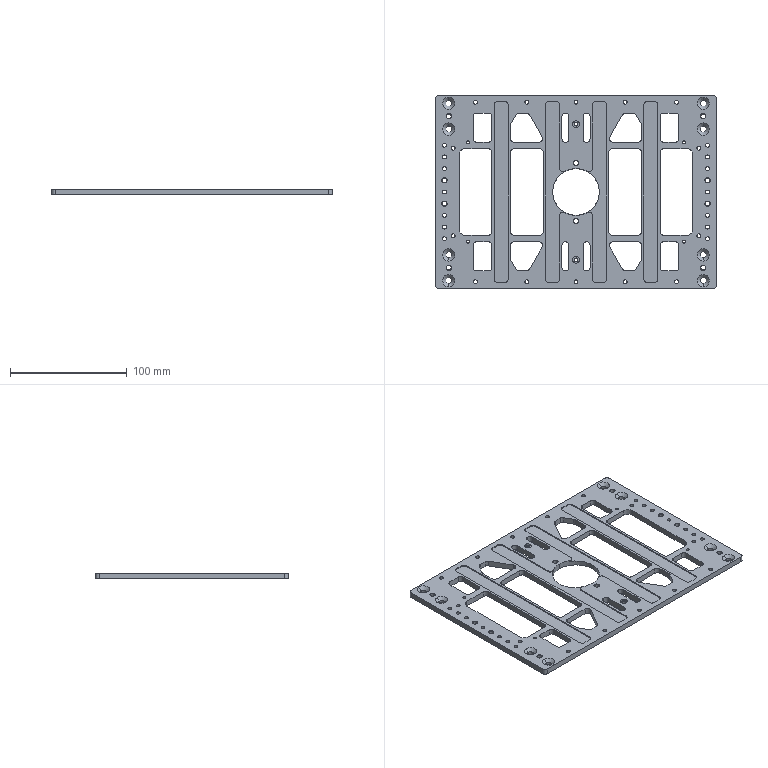NC program | NX | posted with a generic post | part box 240 x 165 x 5 mm
Lines 1759 to 2596 of 12487:
(ZLEVEL_PROFILE_COPY_COPY_1 , TOOL : D4)
N3450 T11 M6
N3452 G54
N3454 G17 G0 G90 X-10. Y-63.427 S9500 M3
N3456 G43 Z30. H11
N3458 Z1.5
N3460 G94 G1 Y-64.672 Z1.435 F1000.
N3462 X-9.86 Y-65.067 Z1.413
N3464 X-9.333 Y-65.475 Z1.378
N3466 X-8.666 Y-65.474 Z1.343
N3468 X-8.251 Y-65.207 Z1.317
N3470 X-8. Y-64.747 Z1.29
N3472 Y-45.253 Z0.268
N3474 X-8.267 Y-44.776 Z0.239
N3476 X-8.741 Y-44.503 Z0.211
N3478 X-9.235 Y-44.497 Z0.185
N3480 X-9.724 Y-44.767 Z0.155
N3482 X-10. Y-45.253 Z0.126
N3484 Y-55. Z-0.385
N3486 Y-64.5 F1800.
N3488 G3 X-9. Y-65.5 R1.
N3490 X-8. Y-64.5 R1.
N3492 G1 Y-45.5
N3494 G3 X-9. Y-44.5 R1.
N3496 X-10. Y-45.5 R1.
N3498 G1 Y-55.
N3500 Y-62.917 Z-0.453
N3502 X-9.983 Y-64.5 Z-0.467
N3504 X-9.955 Y-64.723 Z-0.469
N3506 X-9.921 Y-64.827 Z-0.47
N3508 X-9.782 Y-65.083 Z-0.473
N3510 X-9.691 Y-65.2 Z-0.474
N3512 X-9.501 Y-65.346 Z-0.476
N3514 X-9.316 Y-65.425 Z-0.478
N3516 X-9.063 Y-65.476 Z-0.48
N3518 X-8.881 Y-65.468 Z-0.482
N3520 X-8.635 Y-65.405 Z-0.484
N3522 X-8.47 Y-65.323 Z-0.486
N3524 X-8.336 Y-65.221 Z-0.487
N3526 X-8.233 Y-65.103 Z-0.489
N3528 X-8.127 Y-64.94 Z-0.49
N3530 X-8.076 Y-64.819 Z-0.491
N3532 X-8.039 Y-64.676 Z-0.493
N3534 X-8.017 Y-64.5 Z-0.494
N3536 X-8. Y-62.6 Z-0.511
N3538 Y-47.4 Z-0.643
N3540 X-8.017 Y-45.5 Z-0.66
N3542 X-8.047 Y-45.262 Z-0.662
N3544 X-8.097 Y-45.129 Z-0.663
N3546 X-8.219 Y-44.915 Z-0.665
N3548 X-8.301 Y-44.809 Z-0.666
N3550 X-8.474 Y-44.649 Z-0.668
N3552 X-8.609 Y-44.58 Z-0.67
N3554 X-8.988 Y-44.5 Z-0.673
N3556 X-9.145 Y-44.535 Z-0.674
N3558 X-9.365 Y-44.595 Z-0.676
N3560 X-9.566 Y-44.705 Z-0.678
N3562 X-9.691 Y-44.801 Z-0.68
N3564 X-9.812 Y-44.955 Z-0.682
N3566 X-9.9 Y-45.124 Z-0.683
N3568 X-9.956 Y-45.287 Z-0.685
N3570 X-9.983 Y-45.5 Z-0.687
N3572 X-10. Y-47.083 Z-0.7
N3574 Y-55. Z-0.769
N3576 Y-62.917 Z-0.838
N3578 X-9.983 Y-64.5 Z-0.852
N3580 X-9.955 Y-64.723 Z-0.854
N3582 X-9.921 Y-64.827 Z-0.855
N3584 X-9.782 Y-65.083 Z-0.857
N3586 X-9.691 Y-65.2 Z-0.859
N3588 X-9.501 Y-65.346 Z-0.861
N3590 X-9.316 Y-65.425 Z-0.863
N3592 X-9.063 Y-65.476 Z-0.865
N3594 X-8.881 Y-65.468 Z-0.866
N3596 X-8.635 Y-65.405 Z-0.869
N3598 X-8.47 Y-65.323 Z-0.87
N3600 X-8.336 Y-65.221 Z-0.872
N3602 X-8.233 Y-65.103 Z-0.873
N3604 X-8.127 Y-64.94 Z-0.875
N3606 X-8.076 Y-64.819 Z-0.876
N3608 X-8.039 Y-64.676 Z-0.877
N3610 X-8.017 Y-64.5 Z-0.879
N3612 X-8. Y-62.6 Z-0.895
N3614 Y-47.4 Z-1.028
N3616 X-8.017 Y-45.5 Z-1.044
N3618 X-8.047 Y-45.262 Z-1.046
N3620 X-8.097 Y-45.129 Z-1.047
N3622 X-8.219 Y-44.915 Z-1.05
N3624 X-8.301 Y-44.809 Z-1.051
N3626 X-8.474 Y-44.649 Z-1.053
N3628 X-8.609 Y-44.58 Z-1.054
N3630 X-8.988 Y-44.5 Z-1.058
N3632 X-9.145 Y-44.535 Z-1.059
N3634 X-9.365 Y-44.595 Z-1.061
N3636 X-9.566 Y-44.705 Z-1.063
N3638 X-9.691 Y-44.801 Z-1.064
N3640 X-9.812 Y-44.955 Z-1.066
N3642 X-9.9 Y-45.124 Z-1.068
N3644 X-9.956 Y-45.287 Z-1.069
N3646 X-9.983 Y-45.5 Z-1.071
N3648 X-10. Y-47.083 Z-1.085
N3650 Y-55. Z-1.154
N3652 Y-62.917 Z-1.223
N3654 X-9.983 Y-64.5 Z-1.236
N3656 X-9.955 Y-64.723 Z-1.238
N3658 X-9.921 Y-64.827 Z-1.239
N3660 X-9.782 Y-65.082 Z-1.242
N3662 X-9.691 Y-65.2 Z-1.243
N3664 X-9.501 Y-65.346 Z-1.245
N3666 X-9.316 Y-65.425 Z-1.247
N3668 X-9.063 Y-65.476 Z-1.249
N3670 X-8.881 Y-65.468 Z-1.251
N3672 X-8.635 Y-65.405 Z-1.253
N3674 X-8.47 Y-65.323 Z-1.255
N3676 X-8.336 Y-65.221 Z-1.256
N3678 X-8.233 Y-65.103 Z-1.258
N3680 X-8.127 Y-64.94 Z-1.26
N3682 X-8.076 Y-64.819 Z-1.261
N3684 X-8.039 Y-64.676 Z-1.262
N3686 X-8.017 Y-64.5 Z-1.264
N3688 X-8. Y-62.6 Z-1.28
N3690 Y-47.4 Z-1.412
N3692 X-8.017 Y-45.5 Z-1.429
N3694 X-8.047 Y-45.262 Z-1.431
N3696 X-8.098 Y-45.129 Z-1.432
N3698 X-8.219 Y-44.915 Z-1.434
N3700 X-8.301 Y-44.809 Z-1.435
N3702 X-8.474 Y-44.649 Z-1.438
N3704 X-8.609 Y-44.58 Z-1.439
N3706 X-8.988 Y-44.5 Z-1.442
N3708 X-9.145 Y-44.535 Z-1.444
N3710 X-9.365 Y-44.595 Z-1.446
N3712 X-9.566 Y-44.705 Z-1.448
N3714 X-9.691 Y-44.801 Z-1.449
N3716 X-9.812 Y-44.955 Z-1.451
N3718 X-9.9 Y-45.124 Z-1.452
N3720 X-9.956 Y-45.287 Z-1.454
N3722 X-9.983 Y-45.5 Z-1.456
N3724 X-10. Y-47.083 Z-1.47
N3726 Y-55. Z-1.538
N3728 Y-62.917 Z-1.607
N3730 X-9.983 Y-64.5 Z-1.621
N3732 X-9.955 Y-64.723 Z-1.623
N3734 X-9.921 Y-64.827 Z-1.624
N3736 X-9.783 Y-65.084 Z-1.627
N3738 X-9.691 Y-65.2 Z-1.628
N3740 X-9.497 Y-65.348 Z-1.63
N3742 X-9.316 Y-65.425 Z-1.632
N3744 X-9.062 Y-65.476 Z-1.634
N3746 X-8.881 Y-65.468 Z-1.636
N3748 X-8.635 Y-65.405 Z-1.638
N3750 X-8.47 Y-65.323 Z-1.64
N3752 X-8.336 Y-65.221 Z-1.641
N3754 X-8.233 Y-65.103 Z-1.642
N3756 X-8.127 Y-64.94 Z-1.644
N3758 X-8.076 Y-64.819 Z-1.645
N3760 X-8.039 Y-64.676 Z-1.647
N3762 X-8.017 Y-64.5 Z-1.648
N3764 X-8. Y-62.6 Z-1.665
N3766 Y-47.4 Z-1.797
N3768 X-8.017 Y-45.5 Z-1.813
N3770 X-8.047 Y-45.262 Z-1.815
N3772 X-8.098 Y-45.129 Z-1.817
N3774 X-8.219 Y-44.915 Z-1.819
N3776 X-8.301 Y-44.809 Z-1.82
N3778 X-8.474 Y-44.649 Z-1.822
N3780 X-8.609 Y-44.58 Z-1.823
N3782 X-8.988 Y-44.5 Z-1.827
N3784 X-9.145 Y-44.535 Z-1.828
N3786 X-9.365 Y-44.595 Z-1.83
N3788 X-9.566 Y-44.705 Z-1.832
N3790 X-9.691 Y-44.801 Z-1.834
N3792 X-9.812 Y-44.955 Z-1.835
N3794 X-9.9 Y-45.124 Z-1.837
N3796 X-9.956 Y-45.287 Z-1.839
N3798 X-9.983 Y-45.5 Z-1.84
N3800 X-10. Y-47.083 Z-1.854
N3802 Y-55. Z-1.923
N3804 Y-62.917 Z-1.992
N3806 X-9.983 Y-64.5 Z-2.006
N3808 X-9.955 Y-64.723 Z-2.008
N3810 X-9.921 Y-64.827 Z-2.009
N3812 X-9.783 Y-65.084 Z-2.011
N3814 X-9.691 Y-65.2 Z-2.013
N3816 X-9.497 Y-65.348 Z-2.015
N3818 X-9.316 Y-65.425 Z-2.016
N3820 X-9.062 Y-65.476 Z-2.019
N3822 X-8.881 Y-65.468 Z-2.02
N3824 X-8.635 Y-65.405 Z-2.023
N3826 X-8.47 Y-65.323 Z-2.024
N3828 X-8.336 Y-65.221 Z-2.026
N3830 X-8.233 Y-65.103 Z-2.027
N3832 X-8.127 Y-64.94 Z-2.029
N3834 X-8.076 Y-64.819 Z-2.03
N3836 X-8.039 Y-64.676 Z-2.031
N3838 X-8.017 Y-64.5 Z-2.033
N3840 X-8. Y-62.6 Z-2.049
N3842 Y-47.4 Z-2.181
N3844 X-8.017 Y-45.5 Z-2.198
N3846 X-8.047 Y-45.262 Z-2.2
N3848 X-8.098 Y-45.129 Z-2.201
N3850 X-8.219 Y-44.915 Z-2.204
N3852 X-8.301 Y-44.809 Z-2.205
N3854 X-8.474 Y-44.649 Z-2.207
N3856 X-8.609 Y-44.58 Z-2.208
N3858 X-8.988 Y-44.5 Z-2.211
N3860 X-9.145 Y-44.535 Z-2.213
N3862 X-9.365 Y-44.595 Z-2.215
N3864 X-9.566 Y-44.705 Z-2.217
N3866 X-9.691 Y-44.801 Z-2.218
N3868 X-9.812 Y-44.955 Z-2.22
N3870 X-9.9 Y-45.124 Z-2.222
N3872 X-9.956 Y-45.287 Z-2.223
N3874 X-9.983 Y-45.5 Z-2.225
N3876 X-10. Y-47.083 Z-2.239
N3878 Y-55. Z-2.308
N3880 Y-62.917 Z-2.377
N3882 X-9.983 Y-64.5 Z-2.39
N3884 X-9.955 Y-64.723 Z-2.392
N3886 X-9.921 Y-64.827 Z-2.393
N3888 X-9.783 Y-65.084 Z-2.396
N3890 X-9.691 Y-65.2 Z-2.397
N3892 X-9.497 Y-65.348 Z-2.399
N3894 X-9.316 Y-65.425 Z-2.401
N3896 X-9.062 Y-65.476 Z-2.403
N3898 X-8.881 Y-65.468 Z-2.405
N3900 X-8.635 Y-65.405 Z-2.407
N3902 X-8.47 Y-65.323 Z-2.409
N3904 X-8.336 Y-65.221 Z-2.41
N3906 X-8.233 Y-65.103 Z-2.412
N3908 X-8.127 Y-64.94 Z-2.413
N3910 X-8.076 Y-64.819 Z-2.415
N3912 X-8.039 Y-64.676 Z-2.416
N3914 X-8.017 Y-64.5 Z-2.417
N3916 X-8. Y-62.6 Z-2.434
N3918 Y-47.4 Z-2.566
N3920 X-8.017 Y-45.5 Z-2.583
N3922 X-8.047 Y-45.262 Z-2.585
N3924 X-8.098 Y-45.129 Z-2.586
N3926 X-8.219 Y-44.915 Z-2.588
N3928 X-8.301 Y-44.809 Z-2.589
N3930 X-8.474 Y-44.649 Z-2.591
N3932 X-8.609 Y-44.58 Z-2.593
N3934 X-8.988 Y-44.5 Z-2.596
N3936 X-9.145 Y-44.535 Z-2.597
N3938 X-9.365 Y-44.595 Z-2.599
N3940 X-9.566 Y-44.705 Z-2.601
N3942 X-9.691 Y-44.801 Z-2.603
N3944 X-9.812 Y-44.955 Z-2.605
N3946 X-9.9 Y-45.124 Z-2.606
N3948 X-9.956 Y-45.287 Z-2.608
N3950 X-9.983 Y-45.5 Z-2.61
N3952 X-10. Y-47.083 Z-2.623
N3954 Y-55. Z-2.692
N3956 Y-62.917 Z-2.761
N3958 X-9.983 Y-64.5 Z-2.775
N3960 X-9.955 Y-64.723 Z-2.777
N3962 X-9.921 Y-64.827 Z-2.778
N3964 X-9.783 Y-65.084 Z-2.78
N3966 X-9.691 Y-65.2 Z-2.782
N3968 X-9.498 Y-65.348 Z-2.784
N3970 X-9.316 Y-65.425 Z-2.786
N3972 X-9.062 Y-65.476 Z-2.788
N3974 X-8.881 Y-65.468 Z-2.789
N3976 X-8.635 Y-65.405 Z-2.792
N3978 X-8.47 Y-65.323 Z-2.793
N3980 X-8.336 Y-65.221 Z-2.795
N3982 X-8.233 Y-65.103 Z-2.796
N3984 X-8.127 Y-64.94 Z-2.798
N3986 X-8.076 Y-64.819 Z-2.799
N3988 X-8.039 Y-64.676 Z-2.8
N3990 X-8.017 Y-64.5 Z-2.802
N3992 X-8. Y-62.6 Z-2.819
N3994 Y-47.4 Z-2.951
N3996 X-8.017 Y-45.5 Z-2.967
N3998 X-8.047 Y-45.262 Z-2.969
N4000 X-8.098 Y-45.129 Z-2.971
N4002 X-8.219 Y-44.915 Z-2.973
N4004 X-8.301 Y-44.809 Z-2.974
N4006 X-8.474 Y-44.649 Z-2.976
N4008 X-8.609 Y-44.58 Z-2.977
N4010 X-8.988 Y-44.5 Z-2.981
N4012 X-9.145 Y-44.535 Z-2.982
N4014 X-9.365 Y-44.595 Z-2.984
N4016 X-9.566 Y-44.705 Z-2.986
N4018 X-9.691 Y-44.801 Z-2.988
N4020 X-9.812 Y-44.955 Z-2.989
N4022 X-9.9 Y-45.124 Z-2.991
N4024 X-9.956 Y-45.287 Z-2.992
N4026 X-9.983 Y-45.5 Z-2.994
N4028 X-10. Y-47.083 Z-3.008
N4030 Y-55. Z-3.077
N4032 Y-62.917 Z-3.146
N4034 X-9.983 Y-64.5 Z-3.16
N4036 X-9.955 Y-64.723 Z-3.161
N4038 X-9.921 Y-64.827 Z-3.162
N4040 X-9.783 Y-65.083 Z-3.165
N4042 X-9.691 Y-65.2 Z-3.166
N4044 X-9.498 Y-65.348 Z-3.168
N4046 X-9.316 Y-65.425 Z-3.17
N4048 X-9.062 Y-65.476 Z-3.173
N4050 X-8.881 Y-65.468 Z-3.174
N4052 X-8.635 Y-65.405 Z-3.176
N4054 X-8.47 Y-65.323 Z-3.178
N4056 X-8.336 Y-65.221 Z-3.179
N4058 X-8.233 Y-65.103 Z-3.181
N4060 X-8.127 Y-64.94 Z-3.183
N4062 X-8.076 Y-64.819 Z-3.184
N4064 X-8.039 Y-64.676 Z-3.185
N4066 X-8.017 Y-64.5 Z-3.187
N4068 X-8. Y-62.6 Z-3.203
N4070 Y-47.4 Z-3.335
N4072 X-8.017 Y-45.5 Z-3.352
N4074 X-8.047 Y-45.262 Z-3.354
N4076 X-8.098 Y-45.129 Z-3.355
N4078 X-8.219 Y-44.915 Z-3.357
N4080 X-8.301 Y-44.809 Z-3.359
N4082 X-8.474 Y-44.65 Z-3.361
N4084 X-8.609 Y-44.58 Z-3.362
N4086 X-8.988 Y-44.5 Z-3.365
N4088 X-9.145 Y-44.535 Z-3.367
N4090 X-9.365 Y-44.595 Z-3.369
N4092 X-9.566 Y-44.705 Z-3.371
N4094 X-9.691 Y-44.801 Z-3.372
N4096 X-9.812 Y-44.955 Z-3.374
N4098 X-9.9 Y-45.124 Z-3.376
N4100 X-9.956 Y-45.287 Z-3.377
N4102 X-9.983 Y-45.5 Z-3.379
N4104 X-10. Y-47.083 Z-3.393
N4106 Y-55. Z-3.462
N4108 Y-62.917 Z-3.53
N4110 X-9.983 Y-64.5 Z-3.544
N4112 X-9.955 Y-64.723 Z-3.546
N4114 X-9.921 Y-64.827 Z-3.547
N4116 X-9.783 Y-65.083 Z-3.55
N4118 X-9.691 Y-65.2 Z-3.551
N4120 X-9.498 Y-65.348 Z-3.553
N4122 X-9.316 Y-65.425 Z-3.555
N4124 X-9.062 Y-65.476 Z-3.557
N4126 X-8.881 Y-65.468 Z-3.559
N4128 X-8.635 Y-65.404 Z-3.561
N4130 X-8.47 Y-65.323 Z-3.563
N4132 X-8.336 Y-65.221 Z-3.564
N4134 X-8.233 Y-65.103 Z-3.565
N4136 X-8.127 Y-64.94 Z-3.567
N4138 X-8.076 Y-64.819 Z-3.568
N4140 X-8.039 Y-64.676 Z-3.57
N4142 X-8.017 Y-64.5 Z-3.571
N4144 X-8. Y-62.6 Z-3.588
N4146 Y-47.4 Z-3.72
N4148 X-8.017 Y-45.5 Z-3.736
N4150 X-8.047 Y-45.262 Z-3.739
N4152 X-8.098 Y-45.129 Z-3.74
N4154 X-8.219 Y-44.915 Z-3.742
N4156 X-8.301 Y-44.809 Z-3.743
N4158 X-8.474 Y-44.65 Z-3.745
N4160 X-8.609 Y-44.58 Z-3.747
N4162 X-8.988 Y-44.5 Z-3.75
N4164 X-9.145 Y-44.535 Z-3.751
N4166 X-9.365 Y-44.595 Z-3.753
N4168 X-9.566 Y-44.705 Z-3.755
N4170 X-9.691 Y-44.801 Z-3.757
N4172 X-9.812 Y-44.955 Z-3.758
N4174 X-9.9 Y-45.124 Z-3.76
N4176 X-9.956 Y-45.287 Z-3.762
N4178 X-9.983 Y-45.5 Z-3.764
N4180 X-10. Y-47.083 Z-3.777
N4182 Y-55. Z-3.846
N4184 Y-62.917 Z-3.915
N4186 X-9.983 Y-64.5 Z-3.929
N4188 X-9.955 Y-64.723 Z-3.931
N4190 X-9.921 Y-64.827 Z-3.932
N4192 X-9.783 Y-65.083 Z-3.934
N4194 X-9.691 Y-65.2 Z-3.936
N4196 X-9.498 Y-65.348 Z-3.938
N4198 X-9.316 Y-65.425 Z-3.939
N4200 X-9.062 Y-65.476 Z-3.942
N4202 X-8.881 Y-65.468 Z-3.943
N4204 X-8.635 Y-65.404 Z-3.946
N4206 X-8.47 Y-65.323 Z-3.947
N4208 X-8.337 Y-65.221 Z-3.949
N4210 X-8.233 Y-65.103 Z-3.95
N4212 X-8.127 Y-64.94 Z-3.952
N4214 X-8.076 Y-64.819 Z-3.953
N4216 X-8.039 Y-64.676 Z-3.954
N4218 X-8.017 Y-64.5 Z-3.956
N4220 X-8. Y-62.6 Z-3.972
N4222 Y-47.4 Z-4.105
N4224 X-8.017 Y-45.5 Z-4.121
N4226 X-8.047 Y-45.262 Z-4.123
N4228 X-8.098 Y-45.129 Z-4.124
N4230 X-8.219 Y-44.915 Z-4.127
N4232 X-8.301 Y-44.809 Z-4.128
N4234 X-8.474 Y-44.65 Z-4.13
N4236 X-8.609 Y-44.58 Z-4.131
N4238 X-8.988 Y-44.5 Z-4.135
N4240 X-9.145 Y-44.535 Z-4.136
N4242 X-9.365 Y-44.595 Z-4.138
N4244 X-9.566 Y-44.705 Z-4.14
N4246 X-9.691 Y-44.801 Z-4.141
N4248 X-9.812 Y-44.955 Z-4.143
N4250 X-9.9 Y-45.124 Z-4.145
N4252 X-9.956 Y-45.287 Z-4.146
N4254 X-9.983 Y-45.5 Z-4.148
N4256 X-10. Y-47.083 Z-4.162
N4258 Y-55. Z-4.231
N4260 Y-62.917 Z-4.3
N4262 X-9.983 Y-64.5 Z-4.313
N4264 X-9.955 Y-64.723 Z-4.315
N4266 X-9.921 Y-64.827 Z-4.316
N4268 X-9.783 Y-65.083 Z-4.319
N4270 X-9.691 Y-65.2 Z-4.32
N4272 X-9.498 Y-65.348 Z-4.322
N4274 X-9.316 Y-65.425 Z-4.324
N4276 X-9.062 Y-65.476 Z-4.326
N4278 X-8.881 Y-65.468 Z-4.328
N4280 X-8.635 Y-65.404 Z-4.33
N4282 X-8.47 Y-65.323 Z-4.332
N4284 X-8.337 Y-65.221 Z-4.333
N4286 X-8.233 Y-65.103 Z-4.335
N4288 X-8.127 Y-64.94 Z-4.336
N4290 X-8.076 Y-64.819 Z-4.338
N4292 X-8.039 Y-64.676 Z-4.339
N4294 X-8.017 Y-64.5 Z-4.34
N4296 X-8. Y-62.6 Z-4.357
N4298 Y-47.4 Z-4.489
N4300 X-8.017 Y-45.5 Z-4.506
N4302 X-8.047 Y-45.262 Z-4.508
N4304 X-8.098 Y-45.129 Z-4.509
N4306 X-8.219 Y-44.915 Z-4.511
N4308 X-8.301 Y-44.809 Z-4.512
N4310 X-8.474 Y-44.65 Z-4.514
N4312 X-8.609 Y-44.58 Z-4.516
N4314 X-8.988 Y-44.5 Z-4.519
N4316 X-9.145 Y-44.535 Z-4.521
N4318 X-9.365 Y-44.595 Z-4.523
N4320 X-9.566 Y-44.706 Z-4.525
N4322 X-9.691 Y-44.801 Z-4.526
N4324 X-9.812 Y-44.955 Z-4.528
N4326 X-9.9 Y-45.124 Z-4.529
N4328 X-9.956 Y-45.287 Z-4.531
N4330 X-9.983 Y-45.5 Z-4.533
N4332 X-10. Y-47.083 Z-4.547
N4334 Y-55. Z-4.615
N4336 Y-62.917 Z-4.684
N4338 X-9.983 Y-64.5 Z-4.698
N4340 X-9.955 Y-64.723 Z-4.7
N4342 X-9.921 Y-64.827 Z-4.701
N4344 X-9.783 Y-65.083 Z-4.703
N4346 X-9.691 Y-65.2 Z-4.705
N4348 X-9.498 Y-65.347 Z-4.707
N4350 X-9.316 Y-65.425 Z-4.709
N4352 X-9.062 Y-65.476 Z-4.711
N4354 X-8.881 Y-65.468 Z-4.713
N4356 X-8.635 Y-65.404 Z-4.715
N4358 X-8.47 Y-65.323 Z-4.716
N4360 X-8.337 Y-65.221 Z-4.718
N4362 X-8.233 Y-65.103 Z-4.719
N4364 X-8.127 Y-64.94 Z-4.721
N4366 X-8.076 Y-64.819 Z-4.722
N4368 X-8.039 Y-64.676 Z-4.724
N4370 X-8.017 Y-64.5 Z-4.725
N4372 X-8. Y-62.6 Z-4.742
N4374 Y-47.4 Z-4.874
N4376 X-8.017 Y-45.5 Z-4.89
N4378 X-8.047 Y-45.262 Z-4.892
N4380 X-8.098 Y-45.129 Z-4.894
N4382 X-8.219 Y-44.915 Z-4.896
N4384 X-8.301 Y-44.809 Z-4.897
N4386 X-8.474 Y-44.65 Z-4.899
N4388 X-8.609 Y-44.58 Z-4.9
N4390 X-8.988 Y-44.5 Z-4.904
N4392 X-9.145 Y-44.535 Z-4.905
N4394 X-9.365 Y-44.595 Z-4.907
N4396 X-9.566 Y-44.706 Z-4.909
N4398 X-9.691 Y-44.801 Z-4.911
N4400 X-9.812 Y-44.955 Z-4.912
N4402 X-9.9 Y-45.124 Z-4.914
N4404 X-9.956 Y-45.287 Z-4.916
N4406 X-9.983 Y-45.5 Z-4.917
N4408 X-10. Y-47.083 Z-4.931
N4410 Y-55. Z-5.
N4412 Y-64.5
N4414 G3 X-9. Y-65.5 R1.
N4416 X-8. Y-64.5 R1.
N4418 G1 Y-45.5
N4420 G3 X-9. Y-44.5 R1.
N4422 X-10. Y-45.5 R1.
N4424 G1 Y-55.
N4426 Z-3.5
N4428 G0 Z30.
N4430 X8. Y-63.436
N4432 Z1.5
N4434 G1 Y-64.747 Z1.431 F1000.
N4436 X8.252 Y-65.208 Z1.404
N4438 X8.699 Y-65.485 Z1.376
N4440 X9.225 Y-65.505 Z1.349
N4442 X9.666 Y-65.285 Z1.323
N4444 X10. Y-64.747 Z1.29
N4446 Y-45.253 Z0.268
N4448 X9.724 Y-44.767 Z0.239
N4450 X9.235 Y-44.497 Z0.209
N4452 X8.741 Y-44.503 Z0.184
N4454 X8.267 Y-44.776 Z0.155
N4456 X8. Y-45.253 Z0.126
N4458 Y-55. Z-0.385
N4460 Y-64.5 F1800.
N4462 G3 X9. Y-65.5 R1.
N4464 X10. Y-64.5 R1.
N4466 G1 Y-45.5
N4468 G3 X9. Y-44.5 R1.
N4470 X8. Y-45.5 R1.
N4472 G1 Y-55.
N4474 Y-62.917 Z-0.453
N4476 X8.017 Y-64.5 Z-0.467
N4478 X8.05 Y-64.752 Z-0.469
N4480 X8.104 Y-64.886 Z-0.471
N4482 X8.241 Y-65.113 Z-0.473
N4484 X8.325 Y-65.213 Z-0.474
N4486 X8.498 Y-65.345 Z-0.476
N4488 X8.664 Y-65.418 Z-0.478
N4490 X8.9 Y-65.47 Z-0.48
N4492 X9.054 Y-65.478 Z-0.481
N4494 X9.269 Y-65.444 Z-0.483
N4496 X9.436 Y-65.375 Z-0.485
N4498 X9.619 Y-65.256 Z-0.487
N4500 X9.724 Y-65.16 Z-0.488
N4502 X9.843 Y-65.005 Z-0.49
N4504 X9.91 Y-64.853 Z-0.491
N4506 X9.96 Y-64.682 Z-0.493
N4508 X9.983 Y-64.5 Z-0.494
N4510 X10. Y-62.6 Z-0.511
N4512 Y-47.4 Z-0.643
N4514 X9.983 Y-45.5 Z-0.66
N4516 X9.952 Y-45.258 Z-0.662
N4518 X9.9 Y-45.124 Z-0.663
N4520 X9.769 Y-44.899 Z-0.665
N4522 X9.691 Y-44.801 Z-0.666
N4524 X9.544 Y-44.687 Z-0.668
N4526 X9.365 Y-44.595 Z-0.67
N4528 X8.988 Y-44.5 Z-0.673
N4530 X8.609 Y-44.58 Z-0.677
N4532 X8.464 Y-44.682 Z-0.678
N4534 X8.301 Y-44.809 Z-0.68
N4536 X8.183 Y-44.961 Z-0.682
N4538 X8.097 Y-45.129 Z-0.683
N4540 X8.044 Y-45.292 Z-0.685
N4542 X8.017 Y-45.5 Z-0.687
N4544 X8. Y-47.083 Z-0.7
N4546 Y-55. Z-0.769
N4548 Y-62.917 Z-0.838
N4550 X8.017 Y-64.5 Z-0.852
N4552 X8.05 Y-64.752 Z-0.854
N4554 X8.104 Y-64.886 Z-0.855
N4556 X8.241 Y-65.113 Z-0.858
N4558 X8.325 Y-65.213 Z-0.859
N4560 X8.498 Y-65.345 Z-0.861
N4562 X8.664 Y-65.418 Z-0.862
N4564 X8.9 Y-65.47 Z-0.864
N4566 X9.054 Y-65.478 Z-0.866
N4568 X9.269 Y-65.444 Z-0.868
N4570 X9.436 Y-65.375 Z-0.869
N4572 X9.619 Y-65.256 Z-0.871
N4574 X9.724 Y-65.16 Z-0.873
N4576 X9.843 Y-65.005 Z-0.874
N4578 X9.91 Y-64.853 Z-0.876
N4580 X9.96 Y-64.682 Z-0.877
N4582 X9.983 Y-64.5 Z-0.879
N4584 X10. Y-62.6 Z-0.895
N4586 Y-47.4 Z-1.028
N4588 X9.983 Y-45.5 Z-1.044
N4590 X9.952 Y-45.258 Z-1.046
N4592 X9.9 Y-45.124 Z-1.048
N4594 X9.769 Y-44.899 Z-1.05
N4596 X9.691 Y-44.801 Z-1.051
N4598 X9.544 Y-44.687 Z-1.053
N4600 X9.365 Y-44.595 Z-1.054
N4602 X8.988 Y-44.5 Z-1.058
N4604 X8.609 Y-44.58 Z-1.061
N4606 X8.464 Y-44.682 Z-1.063
N4608 X8.301 Y-44.809 Z-1.065
N4610 X8.183 Y-44.961 Z-1.066
N4612 X8.097 Y-45.129 Z-1.068
N4614 X8.044 Y-45.292 Z-1.069
N4616 X8.017 Y-45.5 Z-1.071
N4618 X8. Y-47.083 Z-1.085
N4620 Y-55. Z-1.154
N4622 Y-62.917 Z-1.223
N4624 X8.017 Y-64.5 Z-1.236
N4626 X8.05 Y-64.752 Z-1.239
N4628 X8.104 Y-64.886 Z-1.24
N4630 X8.241 Y-65.113 Z-1.242
N4632 X8.325 Y-65.213 Z-1.243
N4634 X8.498 Y-65.345 Z-1.245
N4636 X8.664 Y-65.418 Z-1.247
N4638 X8.9 Y-65.47 Z-1.249
N4640 X9.054 Y-65.478 Z-1.25
N4642 X9.269 Y-65.444 Z-1.252
N4644 X9.436 Y-65.375 Z-1.254
N4646 X9.619 Y-65.256 Z-1.256
N4648 X9.724 Y-65.16 Z-1.257
N4650 X9.843 Y-65.005 Z-1.259
N4652 X9.91 Y-64.853 Z-1.26
N4654 X9.96 Y-64.682 Z-1.262
N4656 X9.983 Y-64.5 Z-1.264
N4658 X10. Y-62.6 Z-1.28
N4660 Y-47.4 Z-1.412
N4662 X9.983 Y-45.5 Z-1.429
N4664 X9.952 Y-45.258 Z-1.431
N4666 X9.9 Y-45.124 Z-1.432
N4668 X9.769 Y-44.899 Z-1.434
N4670 X9.691 Y-44.801 Z-1.436
N4672 X9.544 Y-44.687 Z-1.437
N4674 X9.365 Y-44.595 Z-1.439
N4676 X8.988 Y-44.5 Z-1.442
N4678 X8.609 Y-44.58 Z-1.446
N4680 X8.464 Y-44.682 Z-1.447
N4682 X8.301 Y-44.809 Z-1.449
N4684 X8.183 Y-44.961 Z-1.451
N4686 X8.098 Y-45.129 Z-1.453
N4688 X8.044 Y-45.292 Z-1.454
N4690 X8.017 Y-45.5 Z-1.456
N4692 X8. Y-47.083 Z-1.47
N4694 Y-55. Z-1.538
N4696 Y-62.917 Z-1.607
N4698 X8.017 Y-64.5 Z-1.621
N4700 X8.05 Y-64.752 Z-1.623
N4702 X8.104 Y-64.886 Z-1.625
N4704 X8.241 Y-65.113 Z-1.627
N4706 X8.325 Y-65.213 Z-1.628
N4708 X8.498 Y-65.345 Z-1.63
N4710 X8.664 Y-65.418 Z-1.632
N4712 X8.9 Y-65.47 Z-1.634
N4714 X9.054 Y-65.478 Z-1.635
N4716 X9.269 Y-65.444 Z-1.637
N4718 X9.436 Y-65.375 Z-1.639
N4720 X9.619 Y-65.256 Z-1.641
N4722 X9.724 Y-65.16 Z-1.642
N4724 X9.843 Y-65.005 Z-1.644
N4726 X9.91 Y-64.853 Z-1.645
N4728 X9.959 Y-64.682 Z-1.647
N4730 X9.983 Y-64.5 Z-1.648
N4732 X10. Y-62.6 Z-1.665
N4734 Y-47.4 Z-1.797
N4736 X9.983 Y-45.5 Z-1.813
N4738 X9.952 Y-45.258 Z-1.816
N4740 X9.9 Y-45.124 Z-1.817
N4742 X9.769 Y-44.899 Z-1.819
N4744 X9.691 Y-44.801 Z-1.82
N4746 X9.544 Y-44.687 Z-1.822
N4748 X9.365 Y-44.595 Z-1.824
N4750 X8.988 Y-44.5 Z-1.827
N4752 X8.609 Y-44.58 Z-1.83
N4754 X8.464 Y-44.682 Z-1.832
N4756 X8.301 Y-44.809 Z-1.834
N4758 X8.183 Y-44.961 Z-1.835
N4760 X8.098 Y-45.129 Z-1.837
N4762 X8.044 Y-45.292 Z-1.839
N4764 X8.017 Y-45.5 Z-1.84
N4766 X8. Y-47.083 Z-1.854
N4768 Y-55. Z-1.923
N4770 Y-62.917 Z-1.992
N4772 X8.017 Y-64.5 Z-2.006
N4774 X8.05 Y-64.752 Z-2.008
N4776 X8.104 Y-64.886 Z-2.009
N4778 X8.241 Y-65.113 Z-2.012
N4780 X8.325 Y-65.213 Z-2.013
N4782 X8.498 Y-65.345 Z-2.015
N4784 X8.664 Y-65.418 Z-2.016
N4786 X8.9 Y-65.47 Z-2.018
N4788 X9.054 Y-65.478 Z-2.02
N4790 X9.269 Y-65.444 Z-2.022
N4792 X9.436 Y-65.375 Z-2.023
N4794 X9.619 Y-65.256 Z-2.025
N4796 X9.724 Y-65.16 Z-2.026
N4798 X9.843 Y-65.005 Z-2.028
N4800 X9.91 Y-64.853 Z-2.03
N4802 X9.959 Y-64.682 Z-2.031
N4804 X9.983 Y-64.5 Z-2.033
N4806 X10. Y-62.6 Z-2.049
N4808 Y-47.4 Z-2.181
N4810 X9.983 Y-45.5 Z-2.198
N4812 X9.952 Y-45.258 Z-2.2
N4814 X9.9 Y-45.124 Z-2.201
N4816 X9.769 Y-44.899 Z-2.204
N4818 X9.691 Y-44.801 Z-2.205
N4820 X9.544 Y-44.687 Z-2.206
N4822 X9.365 Y-44.595 Z-2.208
N4824 X8.988 Y-44.5 Z-2.212
N4826 X8.609 Y-44.58 Z-2.215
N4828 X8.464 Y-44.682 Z-2.217
N4830 X8.301 Y-44.809 Z-2.218
N4832 X8.183 Y-44.961 Z-2.22
N4834 X8.098 Y-45.129 Z-2.222
N4836 X8.044 Y-45.292 Z-2.223
N4838 X8.017 Y-45.5 Z-2.225
N4840 X8. Y-47.083 Z-2.239
N4842 Y-55. Z-2.308
N4844 Y-62.917 Z-2.377
N4846 X8.017 Y-64.5 Z-2.39
N4848 X8.05 Y-64.752 Z-2.393
N4850 X8.104 Y-64.886 Z-2.394
N4852 X8.241 Y-65.112 Z-2.396
N4854 X8.326 Y-65.213 Z-2.397
N4856 X8.498 Y-65.345 Z-2.399
N4858 X8.664 Y-65.418 Z-2.401
N4860 X8.9 Y-65.47 Z-2.403
N4862 X9.054 Y-65.478 Z-2.404
N4864 X9.269 Y-65.444 Z-2.406
N4866 X9.436 Y-65.375 Z-2.408
N4868 X9.619 Y-65.256 Z-2.41
N4870 X9.724 Y-65.16 Z-2.411
N4872 X9.843 Y-65.005 Z-2.413
N4874 X9.91 Y-64.853 Z-2.414
N4876 X9.959 Y-64.682 Z-2.416
N4878 X9.983 Y-64.5 Z-2.417
N4880 X10. Y-62.6 Z-2.434
N4882 Y-47.4 Z-2.566
N4884 X9.983 Y-45.5 Z-2.583
N4886 X9.952 Y-45.258 Z-2.585
N4888 X9.9 Y-45.124 Z-2.586
N4890 X9.769 Y-44.899 Z-2.588
N4892 X9.691 Y-44.801 Z-2.589
N4894 X9.544 Y-44.687 Z-2.591
N4896 X9.365 Y-44.595 Z-2.593
N4898 X8.988 Y-44.5 Z-2.596
N4900 X8.609 Y-44.58 Z-2.6
N4902 X8.464 Y-44.682 Z-2.601
N4904 X8.301 Y-44.809 Z-2.603
N4906 X8.184 Y-44.961 Z-2.605
N4908 X8.098 Y-45.129 Z-2.606
N4910 X8.044 Y-45.292 Z-2.608
N4912 X8.017 Y-45.5 Z-2.61
N4914 X8. Y-47.083 Z-2.623
N4916 Y-55. Z-2.692
N4918 Y-62.917 Z-2.761
N4920 X8.017 Y-64.5 Z-2.775
N4922 X8.05 Y-64.752 Z-2.777
N4924 X8.104 Y-64.886 Z-2.778
N4926 X8.241 Y-65.112 Z-2.781
N4928 X8.326 Y-65.213 Z-2.782
N4930 X8.498 Y-65.345 Z-2.784
N4932 X8.664 Y-65.418 Z-2.785
N4934 X8.9 Y-65.47 Z-2.788
N4936 X9.054 Y-65.478 Z-2.789
N4938 X9.269 Y-65.444 Z-2.791
N4940 X9.436 Y-65.375 Z-2.792
N4942 X9.619 Y-65.256 Z-2.794
N4944 X9.724 Y-65.16 Z-2.796
N4946 X9.843 Y-65.005 Z-2.797
N4948 X9.91 Y-64.853 Z-2.799
N4950 X9.959 Y-64.682 Z-2.8
N4952 X9.983 Y-64.5 Z-2.802
N4954 X10. Y-62.6 Z-2.819
N4956 Y-47.4 Z-2.951
N4958 X9.983 Y-45.5 Z-2.967
N4960 X9.952 Y-45.258 Z-2.969
N4962 X9.9 Y-45.124 Z-2.971
N4964 X9.769 Y-44.899 Z-2.973
N4966 X9.691 Y-44.801 Z-2.974
N4968 X9.544 Y-44.687 Z-2.976
N4970 X9.365 Y-44.595 Z-2.977
N4972 X8.988 Y-44.5 Z-2.981
N4974 X8.609 Y-44.58 Z-2.984
N4976 X8.464 Y-44.682 Z-2.986
N4978 X8.301 Y-44.809 Z-2.988
N4980 X8.184 Y-44.961 Z-2.989
N4982 X8.098 Y-45.129 Z-2.991
N4984 X8.044 Y-45.292 Z-2.992
N4986 X8.017 Y-45.5 Z-2.994
N4988 X8. Y-47.083 Z-3.008
N4990 Y-55. Z-3.077
N4992 Y-62.917 Z-3.146
N4994 X8.017 Y-64.5 Z-3.16
N4996 X8.05 Y-64.752 Z-3.162
N4998 X8.104 Y-64.886 Z-3.163
N5000 X8.241 Y-65.112 Z-3.165
N5002 X8.326 Y-65.213 Z-3.167
N5004 X8.498 Y-65.345 Z-3.168
N5006 X8.664 Y-65.418 Z-3.17
N5008 X8.9 Y-65.47 Z-3.172
N5010 X9.054 Y-65.478 Z-3.174
N5012 X9.269 Y-65.444 Z-3.175
N5014 X9.436 Y-65.375 Z-3.177
N5016 X9.619 Y-65.256 Z-3.179
N5018 X9.724 Y-65.16 Z-3.18
N5020 X9.843 Y-65.005 Z-3.182
N5022 X9.91 Y-64.852 Z-3.183
N5024 X9.959 Y-64.682 Z-3.185
N5026 X9.983 Y-64.5 Z-3.187
N5028 X10. Y-62.6 Z-3.203
N5030 Y-47.4 Z-3.335
N5032 X9.983 Y-45.5 Z-3.352
N5034 X9.952 Y-45.258 Z-3.354
N5036 X9.9 Y-45.124 Z-3.355
N5038 X9.769 Y-44.899 Z-3.358
N5040 X9.691 Y-44.801 Z-3.359
N5042 X9.544 Y-44.687 Z-3.36
N5044 X9.365 Y-44.595 Z-3.362
N5046 X8.988 Y-44.5 Z-3.365
N5048 X8.609 Y-44.58 Z-3.369
N5050 X8.464 Y-44.682 Z-3.37
N5052 X8.301 Y-44.809 Z-3.372
N5054 X8.184 Y-44.961 Z-3.374
N5056 X8.098 Y-45.129 Z-3.376
N5058 X8.044 Y-45.292 Z-3.377
N5060 X8.017 Y-45.5 Z-3.379
N5062 X8. Y-47.083 Z-3.393
N5064 Y-55. Z-3.462
N5066 Y-62.917 Z-3.53
N5068 X8.017 Y-64.5 Z-3.544
N5070 X8.05 Y-64.752 Z-3.546
N5072 X8.104 Y-64.886 Z-3.548
N5074 X8.241 Y-65.112 Z-3.55
N5076 X8.326 Y-65.213 Z-3.551
N5078 X8.498 Y-65.345 Z-3.553
N5080 X8.664 Y-65.418 Z-3.555
N5082 X8.9 Y-65.47 Z-3.557
N5084 X9.054 Y-65.478 Z-3.558
N5086 X9.269 Y-65.444 Z-3.56
N5088 X9.436 Y-65.375 Z-3.562
N5090 X9.619 Y-65.256 Z-3.564
N5092 X9.724 Y-65.16 Z-3.565
N5094 X9.843 Y-65.005 Z-3.567
N5096 X9.91 Y-64.852 Z-3.568
N5098 X9.959 Y-64.682 Z-3.57
N5100 X9.983 Y-64.5 Z-3.571
N5102 X10. Y-62.6 Z-3.588
N5104 Y-47.4 Z-3.72
N5106 X9.983 Y-45.5 Z-3.736
N5108 X9.952 Y-45.258 Z-3.739
N5110 X9.9 Y-45.124 Z-3.74
N5112 X9.769 Y-44.899 Z-3.742
N5114 X9.691 Y-44.801 Z-3.743
N5116 X9.544 Y-44.687 Z-3.745
N5118 X9.365 Y-44.595 Z-3.747